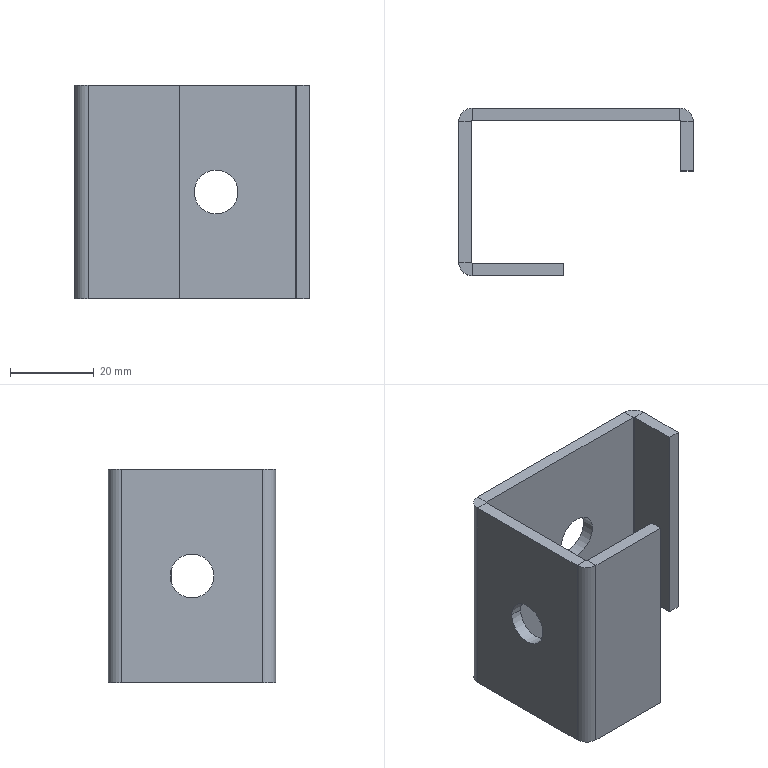Part | SolidWorks | features ICE 2, FlatPattern 1, SMBaseFlange 1, SheetMetal 1 | 1 solid | 34 faces | box 56 x 40 x 51 mm | volume 18577 mm3 | plane 24 | cylinder 10 | commonest cylinder face diameters 10.5 x4 0.4 x3 6.4 x3
STEP:
#1=CARTESIAN_POINT('',(33.75,-3.,30.75));
#2=VERTEX_POINT('',#1);
#3=CARTESIAN_POINT('',(33.75,-3.,20.25));
#4=VERTEX_POINT('',#3);
#5=CARTESIAN_POINT('',(33.75,-3.,25.5));
#6=DIRECTION('',(0.,-1.,0.));
#7=DIRECTION('',(0.,0.,-1.));
#8=AXIS2_PLACEMENT_3D('',#5,#6,#7);
#9=CIRCLE('',#8,5.25);
#10=EDGE_CURVE('',#2,#4,#9,.T.);
#11=ORIENTED_EDGE('',*,*,#10,.T.);
#12=CARTESIAN_POINT('',(33.75,0.,20.25));
#13=VERTEX_POINT('',#12);
#14=CARTESIAN_POINT('',(33.75,-10.,20.25));
#15=DIRECTION('',(0.,1.,0.));
#16=VECTOR('',#15,1000.);
#17=LINE('',#14,#16);
#18=EDGE_CURVE('',#4,#13,#17,.T.);
#19=ORIENTED_EDGE('',*,*,#18,.T.);
#20=CARTESIAN_POINT('',(33.75,0.,30.75));
#21=VERTEX_POINT('',#20);
#22=CARTESIAN_POINT('',(33.75,0.,25.5));
#23=DIRECTION('',(0.,1.,0.));
#24=DIRECTION('',(0.,0.,1.));
#25=AXIS2_PLACEMENT_3D('',#22,#23,#24);
#26=CIRCLE('',#25,5.25);
#27=EDGE_CURVE('',#13,#21,#26,.T.);
#28=ORIENTED_EDGE('',*,*,#27,.T.);
#29=CARTESIAN_POINT('',(33.75,-10.,30.75));
#30=DIRECTION('',(0.,1.,0.));
#31=VECTOR('',#30,1000.);
#32=LINE('',#29,#31);
#33=EDGE_CURVE('',#2,#21,#32,.T.);
#34=ORIENTED_EDGE('',*,*,#33,.F.);
#35=EDGE_LOOP('',(#11,#19,#28,#34));
#36=FACE_OUTER_BOUND('',#35,.T.);
#37=CARTESIAN_POINT('',(33.75,-10.,25.5));
#38=DIRECTION('',(0.,1.,0.));
#39=DIRECTION('',(0.,0.,1.));
#40=AXIS2_PLACEMENT_3D('',#37,#38,#39);
#41=CYLINDRICAL_SURFACE('',#40,5.25);
#42=ADVANCED_FACE('',(#36),#41,.F.);
#43=CARTESIAN_POINT('',(3.,-25.25,25.5));
#44=VERTEX_POINT('',#43);
#45=CARTESIAN_POINT('',(3.,-14.75,25.5));
#46=VERTEX_POINT('',#45);
#47=CARTESIAN_POINT('',(3.,-20.,25.5));
#48=DIRECTION('',(1.,0.,0.));
#49=DIRECTION('',(0.,1.,0.));
#50=AXIS2_PLACEMENT_3D('',#47,#48,#49);
#51=CIRCLE('',#50,5.25);
#52=EDGE_CURVE('',#44,#46,#51,.T.);
#53=ORIENTED_EDGE('',*,*,#52,.T.);
#54=CARTESIAN_POINT('',(0.,-14.75,25.5));
#55=VERTEX_POINT('',#54);
#56=CARTESIAN_POINT('',(10.,-14.75,25.5));
#57=DIRECTION('',(-1.,0.,0.));
#58=VECTOR('',#57,1000.);
#59=LINE('',#56,#58);
#60=EDGE_CURVE('',#46,#55,#59,.T.);
#61=ORIENTED_EDGE('',*,*,#60,.T.);
#62=CARTESIAN_POINT('',(0.,-25.25,25.5));
#63=VERTEX_POINT('',#62);
#64=CARTESIAN_POINT('',(0.,-20.,25.5));
#65=DIRECTION('',(-1.,0.,0.));
#66=DIRECTION('',(0.,-1.,0.));
#67=AXIS2_PLACEMENT_3D('',#64,#65,#66);
#68=CIRCLE('',#67,5.25);
#69=EDGE_CURVE('',#55,#63,#68,.T.);
#70=ORIENTED_EDGE('',*,*,#69,.T.);
#71=CARTESIAN_POINT('',(10.,-25.25,25.5));
#72=DIRECTION('',(-1.,0.,0.));
#73=VECTOR('',#72,1000.);
#74=LINE('',#71,#73);
#75=EDGE_CURVE('',#44,#63,#74,.T.);
#76=ORIENTED_EDGE('',*,*,#75,.F.);
#77=EDGE_LOOP('',(#53,#61,#70,#76));
#78=FACE_OUTER_BOUND('',#77,.T.);
#79=CARTESIAN_POINT('',(10.,-20.,25.5));
#80=DIRECTION('',(-1.,0.,0.));
#81=DIRECTION('',(0.,-1.,0.));
#82=AXIS2_PLACEMENT_3D('',#79,#80,#81);
#83=CYLINDRICAL_SURFACE('',#82,5.25);
#84=ADVANCED_FACE('',(#78),#83,.F.);
#85=CARTESIAN_POINT('',(56.,-3.2,51.));
#86=VERTEX_POINT('',#85);
#87=CARTESIAN_POINT('',(53.,-3.2,51.));
#88=VERTEX_POINT('',#87);
#89=CARTESIAN_POINT('',(56.,-3.2,51.));
#90=DIRECTION('',(-1.,0.,0.));
#91=VECTOR('',#90,1000.);
#92=LINE('',#89,#91);
#93=EDGE_CURVE('',#86,#88,#92,.T.);
#94=ORIENTED_EDGE('',*,*,#93,.F.);
#95=CARTESIAN_POINT('',(52.8,0.,51.));
#96=VERTEX_POINT('',#95);
#97=CARTESIAN_POINT('',(52.8,-3.2,51.));
#98=DIRECTION('',(0.,0.,1.));
#99=DIRECTION('',(-1.,0.,0.));
#100=AXIS2_PLACEMENT_3D('',#97,#98,#99);
#101=CIRCLE('',#100,3.2);
#102=EDGE_CURVE('',#86,#96,#101,.T.);
#103=ORIENTED_EDGE('',*,*,#102,.T.);
#104=CARTESIAN_POINT('',(52.8,-3.,51.));
#105=VERTEX_POINT('',#104);
#106=CARTESIAN_POINT('',(52.8,-3.,51.));
#107=DIRECTION('',(0.,1.,0.));
#108=VECTOR('',#107,1000.);
#109=LINE('',#106,#108);
#110=EDGE_CURVE('',#105,#96,#109,.T.);
#111=ORIENTED_EDGE('',*,*,#110,.F.);
#112=CARTESIAN_POINT('',(52.8,-3.2,51.));
#113=DIRECTION('',(0.,0.,1.));
#114=DIRECTION('',(1.,0.,0.));
#115=AXIS2_PLACEMENT_3D('',#112,#113,#114);
#116=CIRCLE('',#115,0.2);
#117=EDGE_CURVE('',#88,#105,#116,.T.);
#118=ORIENTED_EDGE('',*,*,#117,.F.);
#119=EDGE_LOOP('',(#94,#103,#111,#118));
#120=FACE_OUTER_BOUND('',#119,.T.);
#121=CARTESIAN_POINT('',(56.,-3.2,51.));
#122=DIRECTION('',(0.,0.,1.));
#123=DIRECTION('',(1.,0.,0.));
#124=AXIS2_PLACEMENT_3D('',#121,#122,#123);
#125=PLANE('',#124);
#126=ADVANCED_FACE('',(#120),#125,.T.);
#127=CARTESIAN_POINT('',(56.,-15.,51.));
#128=VERTEX_POINT('',#127);
#129=CARTESIAN_POINT('',(56.,0.,51.));
#130=DIRECTION('',(0.,1.,0.));
#131=VECTOR('',#130,1000.);
#132=LINE('',#129,#131);
#133=EDGE_CURVE('',#128,#86,#132,.T.);
#134=ORIENTED_EDGE('',*,*,#133,.T.);
#135=ORIENTED_EDGE('',*,*,#93,.T.);
#136=CARTESIAN_POINT('',(53.,-15.,51.));
#137=VERTEX_POINT('',#136);
#138=CARTESIAN_POINT('',(53.,0.,51.));
#139=DIRECTION('',(0.,1.,0.));
#140=VECTOR('',#139,1000.);
#141=LINE('',#138,#140);
#142=EDGE_CURVE('',#137,#88,#141,.T.);
#143=ORIENTED_EDGE('',*,*,#142,.F.);
#144=CARTESIAN_POINT('',(56.,-15.,51.));
#145=DIRECTION('',(-1.,0.,0.));
#146=VECTOR('',#145,1000.);
#147=LINE('',#144,#146);
#148=EDGE_CURVE('',#128,#137,#147,.T.);
#149=ORIENTED_EDGE('',*,*,#148,.F.);
#150=EDGE_LOOP('',(#134,#135,#143,#149));
#151=FACE_OUTER_BOUND('',#150,.T.);
#152=CARTESIAN_POINT('',(52.8,-3.,51.));
#153=DIRECTION('',(0.,0.,1.));
#154=DIRECTION('',(1.,0.,0.));
#155=AXIS2_PLACEMENT_3D('',#152,#153,#154);
#156=PLANE('',#155);
#157=ADVANCED_FACE('',(#151),#156,.T.);
#158=CARTESIAN_POINT('',(52.8,0.,0.));
#159=VERTEX_POINT('',#158);
#160=CARTESIAN_POINT('',(52.8,-3.,0.));
#161=VERTEX_POINT('',#160);
#162=CARTESIAN_POINT('',(52.8,0.,0.));
#163=DIRECTION('',(0.,-1.,0.));
#164=VECTOR('',#163,1000.);
#165=LINE('',#162,#164);
#166=EDGE_CURVE('',#159,#161,#165,.T.);
#167=ORIENTED_EDGE('',*,*,#166,.F.);
#168=CARTESIAN_POINT('',(56.,-3.2,0.));
#169=VERTEX_POINT('',#168);
#170=CARTESIAN_POINT('',(52.8,-3.2,0.));
#171=DIRECTION('',(0.,0.,1.));
#172=DIRECTION('',(-1.,0.,0.));
#173=AXIS2_PLACEMENT_3D('',#170,#171,#172);
#174=CIRCLE('',#173,3.2);
#175=EDGE_CURVE('',#169,#159,#174,.T.);
#176=ORIENTED_EDGE('',*,*,#175,.F.);
#177=CARTESIAN_POINT('',(53.,-3.2,0.));
#178=VERTEX_POINT('',#177);
#179=CARTESIAN_POINT('',(53.,-3.2,0.));
#180=DIRECTION('',(1.,0.,0.));
#181=VECTOR('',#180,1000.);
#182=LINE('',#179,#181);
#183=EDGE_CURVE('',#178,#169,#182,.T.);
#184=ORIENTED_EDGE('',*,*,#183,.F.);
#185=CARTESIAN_POINT('',(52.8,-3.2,0.));
#186=DIRECTION('',(0.,0.,1.));
#187=DIRECTION('',(1.,0.,0.));
#188=AXIS2_PLACEMENT_3D('',#185,#186,#187);
#189=CIRCLE('',#188,0.2);
#190=EDGE_CURVE('',#178,#161,#189,.T.);
#191=ORIENTED_EDGE('',*,*,#190,.T.);
#192=EDGE_LOOP('',(#167,#176,#184,#191));
#193=FACE_OUTER_BOUND('',#192,.T.);
#194=CARTESIAN_POINT('',(52.8,0.,0.));
#195=DIRECTION('',(0.,0.,-1.));
#196=DIRECTION('',(-1.,0.,0.));
#197=AXIS2_PLACEMENT_3D('',#194,#195,#196);
#198=PLANE('',#197);
#199=ADVANCED_FACE('',(#193),#198,.T.);
#200=CARTESIAN_POINT('',(3.2,0.,0.));
#201=VERTEX_POINT('',#200);
#202=CARTESIAN_POINT('',(0.,0.,0.));
#203=DIRECTION('',(-1.,0.,0.));
#204=VECTOR('',#203,1000.);
#205=LINE('',#202,#204);
#206=EDGE_CURVE('',#159,#201,#205,.T.);
#207=ORIENTED_EDGE('',*,*,#206,.F.);
#208=ORIENTED_EDGE('',*,*,#166,.T.);
#209=CARTESIAN_POINT('',(3.2,-3.,0.));
#210=VERTEX_POINT('',#209);
#211=CARTESIAN_POINT('',(0.,-3.,0.));
#212=DIRECTION('',(-1.,0.,0.));
#213=VECTOR('',#212,1000.);
#214=LINE('',#211,#213);
#215=EDGE_CURVE('',#161,#210,#214,.T.);
#216=ORIENTED_EDGE('',*,*,#215,.T.);
#217=CARTESIAN_POINT('',(3.2,-3.,0.));
#218=DIRECTION('',(0.,1.,0.));
#219=VECTOR('',#218,1000.);
#220=LINE('',#217,#219);
#221=EDGE_CURVE('',#210,#201,#220,.T.);
#222=ORIENTED_EDGE('',*,*,#221,.T.);
#223=EDGE_LOOP('',(#207,#208,#216,#222));
#224=FACE_OUTER_BOUND('',#223,.T.);
#225=CARTESIAN_POINT('',(53.,-3.2,0.));
#226=DIRECTION('',(0.,0.,-1.));
#227=DIRECTION('',(-1.,0.,0.));
#228=AXIS2_PLACEMENT_3D('',#225,#226,#227);
#229=PLANE('',#228);
#230=ADVANCED_FACE('',(#224),#229,.T.);
#231=CARTESIAN_POINT('',(3.2,0.,51.));
#232=VERTEX_POINT('',#231);
#233=CARTESIAN_POINT('',(3.2,-3.,51.));
#234=VERTEX_POINT('',#233);
#235=CARTESIAN_POINT('',(3.2,0.,51.));
#236=DIRECTION('',(0.,-1.,0.));
#237=VECTOR('',#236,1000.);
#238=LINE('',#235,#237);
#239=EDGE_CURVE('',#232,#234,#238,.T.);
#240=ORIENTED_EDGE('',*,*,#239,.F.);
#241=CARTESIAN_POINT('',(0.,-3.2,51.));
#242=VERTEX_POINT('',#241);
#243=CARTESIAN_POINT('',(3.2,-3.2,51.));
#244=DIRECTION('',(0.,0.,1.));
#245=DIRECTION('',(-1.,0.,0.));
#246=AXIS2_PLACEMENT_3D('',#243,#244,#245);
#247=CIRCLE('',#246,3.2);
#248=EDGE_CURVE('',#232,#242,#247,.T.);
#249=ORIENTED_EDGE('',*,*,#248,.T.);
#250=CARTESIAN_POINT('',(3.,-3.2,51.));
#251=VERTEX_POINT('',#250);
#252=CARTESIAN_POINT('',(3.,-3.2,51.));
#253=DIRECTION('',(-1.,0.,0.));
#254=VECTOR('',#253,1000.);
#255=LINE('',#252,#254);
#256=EDGE_CURVE('',#251,#242,#255,.T.);
#257=ORIENTED_EDGE('',*,*,#256,.F.);
#258=CARTESIAN_POINT('',(3.2,-3.2,51.));
#259=DIRECTION('',(0.,0.,1.));
#260=DIRECTION('',(1.,0.,0.));
#261=AXIS2_PLACEMENT_3D('',#258,#259,#260);
#262=CIRCLE('',#261,0.2);
#263=EDGE_CURVE('',#234,#251,#262,.T.);
#264=ORIENTED_EDGE('',*,*,#263,.F.);
#265=EDGE_LOOP('',(#240,#249,#257,#264));
#266=FACE_OUTER_BOUND('',#265,.T.);
#267=CARTESIAN_POINT('',(3.2,0.,51.));
#268=DIRECTION('',(0.,0.,1.));
#269=DIRECTION('',(1.,0.,0.));
#270=AXIS2_PLACEMENT_3D('',#267,#268,#269);
#271=PLANE('',#270);
#272=ADVANCED_FACE('',(#266),#271,.T.);
#273=CARTESIAN_POINT('',(0.,0.,51.));
#274=DIRECTION('',(-1.,0.,0.));
#275=VECTOR('',#274,1000.);
#276=LINE('',#273,#275);
#277=EDGE_CURVE('',#96,#232,#276,.T.);
#278=ORIENTED_EDGE('',*,*,#277,.T.);
#279=ORIENTED_EDGE('',*,*,#239,.T.);
#280=CARTESIAN_POINT('',(0.,-3.,51.));
#281=DIRECTION('',(-1.,0.,0.));
#282=VECTOR('',#281,1000.);
#283=LINE('',#280,#282);
#284=EDGE_CURVE('',#105,#234,#283,.T.);
#285=ORIENTED_EDGE('',*,*,#284,.F.);
#286=ORIENTED_EDGE('',*,*,#110,.T.);
#287=EDGE_LOOP('',(#278,#279,#285,#286));
#288=FACE_OUTER_BOUND('',#287,.T.);
#289=CARTESIAN_POINT('',(3.,-3.2,51.));
#290=DIRECTION('',(0.,0.,1.));
#291=DIRECTION('',(1.,0.,0.));
#292=AXIS2_PLACEMENT_3D('',#289,#290,#291);
#293=PLANE('',#292);
#294=ADVANCED_FACE('',(#288),#293,.T.);
#295=CARTESIAN_POINT('',(0.,-3.2,0.));
#296=VERTEX_POINT('',#295);
#297=CARTESIAN_POINT('',(3.,-3.2,0.));
#298=VERTEX_POINT('',#297);
#299=CARTESIAN_POINT('',(0.,-3.2,0.));
#300=DIRECTION('',(1.,0.,0.));
#301=VECTOR('',#300,1000.);
#302=LINE('',#299,#301);
#303=EDGE_CURVE('',#296,#298,#302,.T.);
#304=ORIENTED_EDGE('',*,*,#303,.F.);
#305=CARTESIAN_POINT('',(3.2,-3.2,0.));
#306=DIRECTION('',(0.,0.,1.));
#307=DIRECTION('',(-1.,0.,0.));
#308=AXIS2_PLACEMENT_3D('',#305,#306,#307);
#309=CIRCLE('',#308,3.2);
#310=EDGE_CURVE('',#201,#296,#309,.T.);
#311=ORIENTED_EDGE('',*,*,#310,.F.);
#312=ORIENTED_EDGE('',*,*,#221,.F.);
#313=CARTESIAN_POINT('',(3.2,-3.2,0.));
#314=DIRECTION('',(0.,0.,1.));
#315=DIRECTION('',(1.,0.,0.));
#316=AXIS2_PLACEMENT_3D('',#313,#314,#315);
#317=CIRCLE('',#316,0.2);
#318=EDGE_CURVE('',#210,#298,#317,.T.);
#319=ORIENTED_EDGE('',*,*,#318,.T.);
#320=EDGE_LOOP('',(#304,#311,#312,#319));
#321=FACE_OUTER_BOUND('',#320,.T.);
#322=CARTESIAN_POINT('',(0.,-3.2,0.));
#323=DIRECTION('',(0.,0.,-1.));
#324=DIRECTION('',(-1.,0.,0.));
#325=AXIS2_PLACEMENT_3D('',#322,#323,#324);
#326=PLANE('',#325);
#327=ADVANCED_FACE('',(#321),#326,.T.);
#328=CARTESIAN_POINT('',(0.,-36.8,0.));
#329=VERTEX_POINT('',#328);
#330=CARTESIAN_POINT('',(0.,0.,0.));
#331=DIRECTION('',(0.,-1.,0.));
#332=VECTOR('',#331,1000.);
#333=LINE('',#330,#332);
#334=EDGE_CURVE('',#296,#329,#333,.T.);
#335=ORIENTED_EDGE('',*,*,#334,.F.);
#336=ORIENTED_EDGE('',*,*,#303,.T.);
#337=CARTESIAN_POINT('',(3.,-36.8,0.));
#338=VERTEX_POINT('',#337);
#339=CARTESIAN_POINT('',(3.,0.,0.));
#340=DIRECTION('',(0.,-1.,0.));
#341=VECTOR('',#340,1000.);
#342=LINE('',#339,#341);
#343=EDGE_CURVE('',#298,#338,#342,.T.);
#344=ORIENTED_EDGE('',*,*,#343,.T.);
#345=CARTESIAN_POINT('',(3.,-36.8,0.));
#346=DIRECTION('',(-1.,0.,0.));
#347=VECTOR('',#346,1000.);
#348=LINE('',#345,#347);
#349=EDGE_CURVE('',#338,#329,#348,.T.);
#350=ORIENTED_EDGE('',*,*,#349,.T.);
#351=EDGE_LOOP('',(#335,#336,#344,#350));
#352=FACE_OUTER_BOUND('',#351,.T.);
#353=CARTESIAN_POINT('',(3.2,-3.,0.));
#354=DIRECTION('',(0.,0.,-1.));
#355=DIRECTION('',(-1.,0.,0.));
#356=AXIS2_PLACEMENT_3D('',#353,#354,#355);
#357=PLANE('',#356);
#358=ADVANCED_FACE('',(#352),#357,.T.);
#359=CARTESIAN_POINT('',(0.,-36.8,51.));
#360=VERTEX_POINT('',#359);
#361=CARTESIAN_POINT('',(3.,-36.8,51.));
#362=VERTEX_POINT('',#361);
#363=CARTESIAN_POINT('',(0.,-36.8,51.));
#364=DIRECTION('',(1.,0.,0.));
#365=VECTOR('',#364,1000.);
#366=LINE('',#363,#365);
#367=EDGE_CURVE('',#360,#362,#366,.T.);
#368=ORIENTED_EDGE('',*,*,#367,.F.);
#369=CARTESIAN_POINT('',(3.2,-40.,51.));
#370=VERTEX_POINT('',#369);
#371=CARTESIAN_POINT('',(3.2,-36.8,51.));
#372=DIRECTION('',(0.,0.,1.));
#373=DIRECTION('',(-1.,0.,0.));
#374=AXIS2_PLACEMENT_3D('',#371,#372,#373);
#375=CIRCLE('',#374,3.2);
#376=EDGE_CURVE('',#360,#370,#375,.T.);
#377=ORIENTED_EDGE('',*,*,#376,.T.);
#378=CARTESIAN_POINT('',(3.2,-37.,51.));
#379=VERTEX_POINT('',#378);
#380=CARTESIAN_POINT('',(3.2,-37.,51.));
#381=DIRECTION('',(0.,-1.,0.));
#382=VECTOR('',#381,1000.);
#383=LINE('',#380,#382);
#384=EDGE_CURVE('',#379,#370,#383,.T.);
#385=ORIENTED_EDGE('',*,*,#384,.F.);
#386=CARTESIAN_POINT('',(3.2,-36.8,51.));
#387=DIRECTION('',(0.,0.,1.));
#388=DIRECTION('',(1.,0.,0.));
#389=AXIS2_PLACEMENT_3D('',#386,#387,#388);
#390=CIRCLE('',#389,0.2);
#391=EDGE_CURVE('',#362,#379,#390,.T.);
#392=ORIENTED_EDGE('',*,*,#391,.F.);
#393=EDGE_LOOP('',(#368,#377,#385,#392));
#394=FACE_OUTER_BOUND('',#393,.T.);
#395=CARTESIAN_POINT('',(0.,-36.8,51.));
#396=DIRECTION('',(0.,0.,1.));
#397=DIRECTION('',(1.,0.,0.));
#398=AXIS2_PLACEMENT_3D('',#395,#396,#397);
#399=PLANE('',#398);
#400=ADVANCED_FACE('',(#394),#399,.T.);
#401=CARTESIAN_POINT('',(0.,0.,51.));
#402=DIRECTION('',(0.,-1.,0.));
#403=VECTOR('',#402,1000.);
#404=LINE('',#401,#403);
#405=EDGE_CURVE('',#242,#360,#404,.T.);
#406=ORIENTED_EDGE('',*,*,#405,.T.);
#407=ORIENTED_EDGE('',*,*,#367,.T.);
#408=CARTESIAN_POINT('',(3.,0.,51.));
#409=DIRECTION('',(0.,-1.,0.));
#410=VECTOR('',#409,1000.);
#411=LINE('',#408,#410);
#412=EDGE_CURVE('',#251,#362,#411,.T.);
#413=ORIENTED_EDGE('',*,*,#412,.F.);
#414=ORIENTED_EDGE('',*,*,#256,.T.);
#415=EDGE_LOOP('',(#406,#407,#413,#414));
#416=FACE_OUTER_BOUND('',#415,.T.);
#417=CARTESIAN_POINT('',(3.2,-37.,51.));
#418=DIRECTION('',(0.,0.,1.));
#419=DIRECTION('',(1.,0.,0.));
#420=AXIS2_PLACEMENT_3D('',#417,#418,#419);
#421=PLANE('',#420);
#422=ADVANCED_FACE('',(#416),#421,.T.);
#423=CARTESIAN_POINT('',(3.2,-40.,0.));
#424=VERTEX_POINT('',#423);
#425=CARTESIAN_POINT('',(3.2,-37.,0.));
#426=VERTEX_POINT('',#425);
#427=CARTESIAN_POINT('',(3.2,-40.,0.));
#428=DIRECTION('',(0.,1.,0.));
#429=VECTOR('',#428,1000.);
#430=LINE('',#427,#429);
#431=EDGE_CURVE('',#424,#426,#430,.T.);
#432=ORIENTED_EDGE('',*,*,#431,.F.);
#433=CARTESIAN_POINT('',(3.2,-36.8,0.));
#434=DIRECTION('',(0.,0.,1.));
#435=DIRECTION('',(-1.,0.,0.));
#436=AXIS2_PLACEMENT_3D('',#433,#434,#435);
#437=CIRCLE('',#436,3.2);
#438=EDGE_CURVE('',#329,#424,#437,.T.);
#439=ORIENTED_EDGE('',*,*,#438,.F.);
#440=ORIENTED_EDGE('',*,*,#349,.F.);
#441=CARTESIAN_POINT('',(3.2,-36.8,0.));
#442=DIRECTION('',(0.,0.,1.));
#443=DIRECTION('',(1.,0.,0.));
#444=AXIS2_PLACEMENT_3D('',#441,#442,#443);
#445=CIRCLE('',#444,0.2);
#446=EDGE_CURVE('',#338,#426,#445,.T.);
#447=ORIENTED_EDGE('',*,*,#446,.T.);
#448=EDGE_LOOP('',(#432,#439,#440,#447));
#449=FACE_OUTER_BOUND('',#448,.T.);
#450=CARTESIAN_POINT('',(3.2,-40.,0.));
#451=DIRECTION('',(0.,0.,-1.));
#452=DIRECTION('',(-1.,0.,0.));
#453=AXIS2_PLACEMENT_3D('',#450,#451,#452);
#454=PLANE('',#453);
#455=ADVANCED_FACE('',(#449),#454,.T.);
#456=CARTESIAN_POINT('',(25.,-40.,0.));
#457=VERTEX_POINT('',#456);
#458=CARTESIAN_POINT('',(0.,-40.,0.));
#459=DIRECTION('',(1.,0.,0.));
#460=VECTOR('',#459,1000.);
#461=LINE('',#458,#460);
#462=EDGE_CURVE('',#424,#457,#461,.T.);
#463=ORIENTED_EDGE('',*,*,#462,.F.);
#464=ORIENTED_EDGE('',*,*,#431,.T.);
#465=CARTESIAN_POINT('',(25.,-37.,0.));
#466=VERTEX_POINT('',#465);
#467=CARTESIAN_POINT('',(0.,-37.,0.));
#468=DIRECTION('',(1.,0.,0.));
#469=VECTOR('',#468,1000.);
#470=LINE('',#467,#469);
#471=EDGE_CURVE('',#426,#466,#470,.T.);
#472=ORIENTED_EDGE('',*,*,#471,.T.);
#473=CARTESIAN_POINT('',(25.,-37.,0.));
#474=DIRECTION('',(0.,-1.,0.));
#475=VECTOR('',#474,1000.);
#476=LINE('',#473,#475);
#477=EDGE_CURVE('',#466,#457,#476,.T.);
#478=ORIENTED_EDGE('',*,*,#477,.T.);
#479=EDGE_LOOP('',(#463,#464,#472,#478));
#480=FACE_OUTER_BOUND('',#479,.T.);
#481=CARTESIAN_POINT('',(3.,-36.8,0.));
#482=DIRECTION('',(0.,0.,-1.));
#483=DIRECTION('',(-1.,0.,0.));
#484=AXIS2_PLACEMENT_3D('',#481,#482,#483);
#485=PLANE('',#484);
#486=ADVANCED_FACE('',(#480),#485,.T.);
#487=ORIENTED_EDGE('',*,*,#462,.T.);
#488=CARTESIAN_POINT('',(25.,-40.,51.));
#489=VERTEX_POINT('',#488);
#490=CARTESIAN_POINT('',(25.,-40.,51.));
#491=DIRECTION('',(0.,0.,-1.));
#492=VECTOR('',#491,1000.);
#493=LINE('',#490,#492);
#494=EDGE_CURVE('',#489,#457,#493,.T.);
#495=ORIENTED_EDGE('',*,*,#494,.F.);
#496=CARTESIAN_POINT('',(0.,-40.,51.));
#497=DIRECTION('',(1.,0.,0.));
#498=VECTOR('',#497,1000.);
#499=LINE('',#496,#498);
#500=EDGE_CURVE('',#370,#489,#499,.T.);
#501=ORIENTED_EDGE('',*,*,#500,.F.);
#502=CARTESIAN_POINT('',(3.2,-40.,51.));
#503=DIRECTION('',(0.,0.,-1.));
#504=VECTOR('',#503,1000.);
#505=LINE('',#502,#504);
#506=EDGE_CURVE('',#370,#424,#505,.T.);
#507=ORIENTED_EDGE('',*,*,#506,.T.);
#508=EDGE_LOOP('',(#487,#495,#501,#507));
#509=FACE_OUTER_BOUND('',#508,.T.);
#510=CARTESIAN_POINT('',(0.,-40.,51.));
#511=DIRECTION('',(0.,1.,0.));
#512=DIRECTION('',(0.,0.,1.));
#513=AXIS2_PLACEMENT_3D('',#510,#511,#512);
#514=PLANE('',#513);
#515=ADVANCED_FACE('',(#509),#514,.F.);
#516=ORIENTED_EDGE('',*,*,#477,.F.);
#517=CARTESIAN_POINT('',(25.,-37.,51.));
#518=VERTEX_POINT('',#517);
#519=CARTESIAN_POINT('',(25.,-37.,51.));
#520=DIRECTION('',(0.,0.,-1.));
#521=VECTOR('',#520,1000.);
#522=LINE('',#519,#521);
#523=EDGE_CURVE('',#518,#466,#522,.T.);
#524=ORIENTED_EDGE('',*,*,#523,.F.);
#525=CARTESIAN_POINT('',(25.,-37.,51.));
#526=DIRECTION('',(0.,-1.,0.));
#527=VECTOR('',#526,1000.);
#528=LINE('',#525,#527);
#529=EDGE_CURVE('',#518,#489,#528,.T.);
#530=ORIENTED_EDGE('',*,*,#529,.T.);
#531=ORIENTED_EDGE('',*,*,#494,.T.);
#532=EDGE_LOOP('',(#516,#524,#530,#531));
#533=FACE_OUTER_BOUND('',#532,.T.);
#534=CARTESIAN_POINT('',(25.,-37.,51.));
#535=DIRECTION('',(1.,0.,0.));
#536=DIRECTION('',(0.,0.,-1.));
#537=AXIS2_PLACEMENT_3D('',#534,#535,#536);
#538=PLANE('',#537);
#539=ADVANCED_FACE('',(#533),#538,.T.);
#540=ORIENTED_EDGE('',*,*,#471,.F.);
#541=CARTESIAN_POINT('',(3.2,-37.,51.));
#542=DIRECTION('',(0.,0.,-1.));
#543=VECTOR('',#542,1000.);
#544=LINE('',#541,#543);
#545=EDGE_CURVE('',#379,#426,#544,.T.);
#546=ORIENTED_EDGE('',*,*,#545,.F.);
#547=CARTESIAN_POINT('',(0.,-37.,51.));
#548=DIRECTION('',(1.,0.,0.));
#549=VECTOR('',#548,1000.);
#550=LINE('',#547,#549);
#551=EDGE_CURVE('',#379,#518,#550,.T.);
#552=ORIENTED_EDGE('',*,*,#551,.T.);
#553=ORIENTED_EDGE('',*,*,#523,.T.);
#554=EDGE_LOOP('',(#540,#546,#552,#553));
#555=FACE_OUTER_BOUND('',#554,.T.);
#556=CARTESIAN_POINT('',(0.,-37.,51.));
#557=DIRECTION('',(0.,1.,0.));
#558=DIRECTION('',(0.,0.,1.));
#559=AXIS2_PLACEMENT_3D('',#556,#557,#558);
#560=PLANE('',#559);
#561=ADVANCED_FACE('',(#555),#560,.T.);
#562=ORIENTED_EDGE('',*,*,#446,.F.);
#563=CARTESIAN_POINT('',(3.,-36.8,51.));
#564=DIRECTION('',(0.,0.,-1.));
#565=VECTOR('',#564,1000.);
#566=LINE('',#563,#565);
#567=EDGE_CURVE('',#362,#338,#566,.T.);
#568=ORIENTED_EDGE('',*,*,#567,.F.);
#569=ORIENTED_EDGE('',*,*,#391,.T.);
#570=ORIENTED_EDGE('',*,*,#545,.T.);
#571=EDGE_LOOP('',(#562,#568,#569,#570));
#572=FACE_OUTER_BOUND('',#571,.T.);
#573=CARTESIAN_POINT('',(3.2,-36.8,51.));
#574=DIRECTION('',(0.,0.,-1.));
#575=DIRECTION('',(-1.,0.,0.));
#576=AXIS2_PLACEMENT_3D('',#573,#574,#575);
#577=CYLINDRICAL_SURFACE('',#576,0.2);
#578=ADVANCED_FACE('',(#572),#577,.F.);
#579=ORIENTED_EDGE('',*,*,#52,.F.);
#580=CARTESIAN_POINT('',(3.,-20.,25.5));
#581=DIRECTION('',(1.,0.,0.));
#582=DIRECTION('',(0.,1.,0.));
#583=AXIS2_PLACEMENT_3D('',#580,#581,#582);
#584=CIRCLE('',#583,5.25);
#585=EDGE_CURVE('',#46,#44,#584,.T.);
#586=ORIENTED_EDGE('',*,*,#585,.F.);
#587=EDGE_LOOP('',(#579,#586));
#588=FACE_BOUND('',#587,.T.);
#589=ORIENTED_EDGE('',*,*,#343,.F.);
#590=CARTESIAN_POINT('',(3.,-3.2,51.));
#591=DIRECTION('',(0.,0.,-1.));
#592=VECTOR('',#591,1000.);
#593=LINE('',#590,#592);
#594=EDGE_CURVE('',#251,#298,#593,.T.);
#595=ORIENTED_EDGE('',*,*,#594,.F.);
#596=ORIENTED_EDGE('',*,*,#412,.T.);
#597=ORIENTED_EDGE('',*,*,#567,.T.);
#598=EDGE_LOOP('',(#589,#595,#596,#597));
#599=FACE_OUTER_BOUND('',#598,.T.);
#600=CARTESIAN_POINT('',(3.,0.,51.));
#601=DIRECTION('',(1.,0.,0.));
#602=DIRECTION('',(0.,1.,0.));
#603=AXIS2_PLACEMENT_3D('',#600,#601,#602);
#604=PLANE('',#603);
#605=ADVANCED_FACE('',(#588,#599),#604,.T.);
#606=ORIENTED_EDGE('',*,*,#318,.F.);
#607=CARTESIAN_POINT('',(3.2,-3.,51.));
#608=DIRECTION('',(0.,0.,-1.));
#609=VECTOR('',#608,1000.);
#610=LINE('',#607,#609);
#611=EDGE_CURVE('',#234,#210,#610,.T.);
#612=ORIENTED_EDGE('',*,*,#611,.F.);
#613=ORIENTED_EDGE('',*,*,#263,.T.);
#614=ORIENTED_EDGE('',*,*,#594,.T.);
#615=EDGE_LOOP('',(#606,#612,#613,#614));
#616=FACE_OUTER_BOUND('',#615,.T.);
#617=CARTESIAN_POINT('',(3.2,-3.2,51.));
#618=DIRECTION('',(0.,0.,-1.));
#619=DIRECTION('',(-1.,0.,0.));
#620=AXIS2_PLACEMENT_3D('',#617,#618,#619);
#621=CYLINDRICAL_SURFACE('',#620,0.2);
#622=ADVANCED_FACE('',(#616),#621,.F.);
#623=ORIENTED_EDGE('',*,*,#10,.F.);
#624=CARTESIAN_POINT('',(33.75,-3.,25.5));
#625=DIRECTION('',(0.,-1.,0.));
#626=DIRECTION('',(0.,0.,-1.));
#627=AXIS2_PLACEMENT_3D('',#624,#625,#626);
#628=CIRCLE('',#627,5.25);
#629=EDGE_CURVE('',#4,#2,#628,.T.);
#630=ORIENTED_EDGE('',*,*,#629,.F.);
#631=EDGE_LOOP('',(#623,#630));
#632=FACE_BOUND('',#631,.T.);
#633=ORIENTED_EDGE('',*,*,#215,.F.);
#634=CARTESIAN_POINT('',(52.8,-3.,51.));
#635=DIRECTION('',(0.,0.,-1.));
#636=VECTOR('',#635,1000.);
#637=LINE('',#634,#636);
#638=EDGE_CURVE('',#105,#161,#637,.T.);
#639=ORIENTED_EDGE('',*,*,#638,.F.);
#640=ORIENTED_EDGE('',*,*,#284,.T.);
#641=ORIENTED_EDGE('',*,*,#611,.T.);
#642=EDGE_LOOP('',(#633,#639,#640,#641));
#643=FACE_OUTER_BOUND('',#642,.T.);
#644=CARTESIAN_POINT('',(0.,-3.,51.));
#645=DIRECTION('',(0.,-1.,0.));
#646=DIRECTION('',(0.,0.,-1.));
#647=AXIS2_PLACEMENT_3D('',#644,#645,#646);
#648=PLANE('',#647);
#649=ADVANCED_FACE('',(#632,#643),#648,.T.);
#650=ORIENTED_EDGE('',*,*,#190,.F.);
#651=CARTESIAN_POINT('',(53.,-3.2,51.));
#652=DIRECTION('',(0.,0.,-1.));
#653=VECTOR('',#652,1000.);
#654=LINE('',#651,#653);
#655=EDGE_CURVE('',#88,#178,#654,.T.);
#656=ORIENTED_EDGE('',*,*,#655,.F.);
#657=ORIENTED_EDGE('',*,*,#117,.T.);
#658=ORIENTED_EDGE('',*,*,#638,.T.);
#659=EDGE_LOOP('',(#650,#656,#657,#658));
#660=FACE_OUTER_BOUND('',#659,.T.);
#661=CARTESIAN_POINT('',(52.8,-3.2,51.));
#662=DIRECTION('',(0.,0.,-1.));
#663=DIRECTION('',(-1.,0.,0.));
#664=AXIS2_PLACEMENT_3D('',#661,#662,#663);
#665=CYLINDRICAL_SURFACE('',#664,0.2);
#666=ADVANCED_FACE('',(#660),#665,.F.);
#667=CARTESIAN_POINT('',(53.,-15.,0.));
#668=VERTEX_POINT('',#667);
#669=CARTESIAN_POINT('',(53.,0.,0.));
#670=DIRECTION('',(0.,1.,0.));
#671=VECTOR('',#670,1000.);
#672=LINE('',#669,#671);
#673=EDGE_CURVE('',#668,#178,#672,.T.);
#674=ORIENTED_EDGE('',*,*,#673,.F.);
#675=CARTESIAN_POINT('',(53.,-15.,51.));
#676=DIRECTION('',(0.,0.,-1.));
#677=VECTOR('',#676,1000.);
#678=LINE('',#675,#677);
#679=EDGE_CURVE('',#137,#668,#678,.T.);
#680=ORIENTED_EDGE('',*,*,#679,.F.);
#681=ORIENTED_EDGE('',*,*,#142,.T.);
#682=ORIENTED_EDGE('',*,*,#655,.T.);
#683=EDGE_LOOP('',(#674,#680,#681,#682));
#684=FACE_OUTER_BOUND('',#683,.T.);
#685=CARTESIAN_POINT('',(53.,0.,51.));
#686=DIRECTION('',(-1.,0.,0.));
#687=DIRECTION('',(0.,0.,1.));
#688=AXIS2_PLACEMENT_3D('',#685,#686,#687);
#689=PLANE('',#688);
#690=ADVANCED_FACE('',(#684),#689,.T.);
#691=CARTESIAN_POINT('',(56.,-15.,0.));
#692=VERTEX_POINT('',#691);
#693=CARTESIAN_POINT('',(56.,-15.,0.));
#694=DIRECTION('',(-1.,0.,0.));
#695=VECTOR('',#694,1000.);
#696=LINE('',#693,#695);
#697=EDGE_CURVE('',#692,#668,#696,.T.);
#698=ORIENTED_EDGE('',*,*,#697,.F.);
#699=CARTESIAN_POINT('',(56.,-15.,51.));
#700=DIRECTION('',(0.,0.,-1.));
#701=VECTOR('',#700,1000.);
#702=LINE('',#699,#701);
#703=EDGE_CURVE('',#128,#692,#702,.T.);
#704=ORIENTED_EDGE('',*,*,#703,.F.);
#705=ORIENTED_EDGE('',*,*,#148,.T.);
#706=ORIENTED_EDGE('',*,*,#679,.T.);
#707=EDGE_LOOP('',(#698,#704,#705,#706));
#708=FACE_OUTER_BOUND('',#707,.T.);
#709=CARTESIAN_POINT('',(56.,-15.,51.));
#710=DIRECTION('',(0.,-1.,0.));
#711=DIRECTION('',(0.,0.,-1.));
#712=AXIS2_PLACEMENT_3D('',#709,#710,#711);
#713=PLANE('',#712);
#714=ADVANCED_FACE('',(#708),#713,.T.);
#715=CARTESIAN_POINT('',(56.,0.,0.));
#716=DIRECTION('',(0.,1.,0.));
#717=VECTOR('',#716,1000.);
#718=LINE('',#715,#717);
#719=EDGE_CURVE('',#692,#169,#718,.T.);
#720=ORIENTED_EDGE('',*,*,#719,.T.);
#721=CARTESIAN_POINT('',(56.,-3.2,51.));
#722=DIRECTION('',(0.,0.,-1.));
#723=VECTOR('',#722,1000.);
#724=LINE('',#721,#723);
#725=EDGE_CURVE('',#86,#169,#724,.T.);
#726=ORIENTED_EDGE('',*,*,#725,.F.);
#727=ORIENTED_EDGE('',*,*,#133,.F.);
#728=ORIENTED_EDGE('',*,*,#703,.T.);
#729=EDGE_LOOP('',(#720,#726,#727,#728));
#730=FACE_OUTER_BOUND('',#729,.T.);
#731=CARTESIAN_POINT('',(56.,0.,51.));
#732=DIRECTION('',(-1.,0.,0.));
#733=DIRECTION('',(0.,0.,1.));
#734=AXIS2_PLACEMENT_3D('',#731,#732,#733);
#735=PLANE('',#734);
#736=ADVANCED_FACE('',(#730),#735,.F.);
#737=ORIENTED_EDGE('',*,*,#175,.T.);
#738=CARTESIAN_POINT('',(52.8,0.,51.));
#739=DIRECTION('',(0.,0.,-1.));
#740=VECTOR('',#739,1000.);
#741=LINE('',#738,#740);
#742=EDGE_CURVE('',#96,#159,#741,.T.);
#743=ORIENTED_EDGE('',*,*,#742,.F.);
#744=ORIENTED_EDGE('',*,*,#102,.F.);
#745=ORIENTED_EDGE('',*,*,#725,.T.);
#746=EDGE_LOOP('',(#737,#743,#744,#745));
#747=FACE_OUTER_BOUND('',#746,.T.);
#748=CARTESIAN_POINT('',(52.8,-3.2,51.));
#749=DIRECTION('',(0.,0.,-1.));
#750=DIRECTION('',(-1.,0.,0.));
#751=AXIS2_PLACEMENT_3D('',#748,#749,#750);
#752=CYLINDRICAL_SURFACE('',#751,3.2);
#753=ADVANCED_FACE('',(#747),#752,.T.);
#754=CARTESIAN_POINT('',(33.75,0.,25.5));
#755=DIRECTION('',(0.,1.,0.));
#756=DIRECTION('',(0.,0.,1.));
#757=AXIS2_PLACEMENT_3D('',#754,#755,#756);
#758=CIRCLE('',#757,5.25);
#759=EDGE_CURVE('',#21,#13,#758,.T.);
#760=ORIENTED_EDGE('',*,*,#759,.F.);
#761=ORIENTED_EDGE('',*,*,#27,.F.);
#762=EDGE_LOOP('',(#760,#761));
#763=FACE_BOUND('',#762,.T.);
#764=ORIENTED_EDGE('',*,*,#206,.T.);
#765=CARTESIAN_POINT('',(3.2,0.,51.));
#766=DIRECTION('',(0.,0.,-1.));
#767=VECTOR('',#766,1000.);
#768=LINE('',#765,#767);
#769=EDGE_CURVE('',#232,#201,#768,.T.);
#770=ORIENTED_EDGE('',*,*,#769,.F.);
#771=ORIENTED_EDGE('',*,*,#277,.F.);
#772=ORIENTED_EDGE('',*,*,#742,.T.);
#773=EDGE_LOOP('',(#764,#770,#771,#772));
#774=FACE_OUTER_BOUND('',#773,.T.);
#775=CARTESIAN_POINT('',(0.,0.,51.));
#776=DIRECTION('',(0.,-1.,0.));
#777=DIRECTION('',(0.,0.,-1.));
#778=AXIS2_PLACEMENT_3D('',#775,#776,#777);
#779=PLANE('',#778);
#780=ADVANCED_FACE('',(#763,#774),#779,.F.);
#781=ORIENTED_EDGE('',*,*,#310,.T.);
#782=CARTESIAN_POINT('',(0.,-3.2,51.));
#783=DIRECTION('',(0.,0.,-1.));
#784=VECTOR('',#783,1000.);
#785=LINE('',#782,#784);
#786=EDGE_CURVE('',#242,#296,#785,.T.);
#787=ORIENTED_EDGE('',*,*,#786,.F.);
#788=ORIENTED_EDGE('',*,*,#248,.F.);
#789=ORIENTED_EDGE('',*,*,#769,.T.);
#790=EDGE_LOOP('',(#781,#787,#788,#789));
#791=FACE_OUTER_BOUND('',#790,.T.);
#792=CARTESIAN_POINT('',(3.2,-3.2,51.));
#793=DIRECTION('',(0.,0.,-1.));
#794=DIRECTION('',(-1.,0.,0.));
#795=AXIS2_PLACEMENT_3D('',#792,#793,#794);
#796=CYLINDRICAL_SURFACE('',#795,3.2);
#797=ADVANCED_FACE('',(#791),#796,.T.);
#798=CARTESIAN_POINT('',(0.,-20.,25.5));
#799=DIRECTION('',(-1.,0.,0.));
#800=DIRECTION('',(0.,-1.,0.));
#801=AXIS2_PLACEMENT_3D('',#798,#799,#800);
#802=CIRCLE('',#801,5.25);
#803=EDGE_CURVE('',#63,#55,#802,.T.);
#804=ORIENTED_EDGE('',*,*,#803,.F.);
#805=ORIENTED_EDGE('',*,*,#69,.F.);
#806=EDGE_LOOP('',(#804,#805));
#807=FACE_BOUND('',#806,.T.);
#808=ORIENTED_EDGE('',*,*,#334,.T.);
#809=CARTESIAN_POINT('',(0.,-36.8,51.));
#810=DIRECTION('',(0.,0.,-1.));
#811=VECTOR('',#810,1000.);
#812=LINE('',#809,#811);
#813=EDGE_CURVE('',#360,#329,#812,.T.);
#814=ORIENTED_EDGE('',*,*,#813,.F.);
#815=ORIENTED_EDGE('',*,*,#405,.F.);
#816=ORIENTED_EDGE('',*,*,#786,.T.);
#817=EDGE_LOOP('',(#808,#814,#815,#816));
#818=FACE_OUTER_BOUND('',#817,.T.);
#819=CARTESIAN_POINT('',(0.,0.,51.));
#820=DIRECTION('',(1.,0.,0.));
#821=DIRECTION('',(0.,1.,0.));
#822=AXIS2_PLACEMENT_3D('',#819,#820,#821);
#823=PLANE('',#822);
#824=ADVANCED_FACE('',(#807,#818),#823,.F.);
#825=ORIENTED_EDGE('',*,*,#438,.T.);
#826=ORIENTED_EDGE('',*,*,#506,.F.);
#827=ORIENTED_EDGE('',*,*,#376,.F.);
#828=ORIENTED_EDGE('',*,*,#813,.T.);
#829=EDGE_LOOP('',(#825,#826,#827,#828));
#830=FACE_OUTER_BOUND('',#829,.T.);
#831=CARTESIAN_POINT('',(3.2,-36.8,51.));
#832=DIRECTION('',(0.,0.,-1.));
#833=DIRECTION('',(-1.,0.,0.));
#834=AXIS2_PLACEMENT_3D('',#831,#832,#833);
#835=CYLINDRICAL_SURFACE('',#834,3.2);
#836=ADVANCED_FACE('',(#830),#835,.T.);
#837=ORIENTED_EDGE('',*,*,#500,.T.);
#838=ORIENTED_EDGE('',*,*,#529,.F.);
#839=ORIENTED_EDGE('',*,*,#551,.F.);
#840=ORIENTED_EDGE('',*,*,#384,.T.);
#841=EDGE_LOOP('',(#837,#838,#839,#840));
#842=FACE_OUTER_BOUND('',#841,.T.);
#843=CARTESIAN_POINT('',(3.2,-36.8,51.));
#844=DIRECTION('',(0.,0.,1.));
#845=DIRECTION('',(1.,0.,0.));
#846=AXIS2_PLACEMENT_3D('',#843,#844,#845);
#847=PLANE('',#846);
#848=ADVANCED_FACE('',(#842),#847,.T.);
#849=ORIENTED_EDGE('',*,*,#673,.T.);
#850=ORIENTED_EDGE('',*,*,#183,.T.);
#851=ORIENTED_EDGE('',*,*,#719,.F.);
#852=ORIENTED_EDGE('',*,*,#697,.T.);
#853=EDGE_LOOP('',(#849,#850,#851,#852));
#854=FACE_OUTER_BOUND('',#853,.T.);
#855=CARTESIAN_POINT('',(3.2,-36.8,0.));
#856=DIRECTION('',(0.,0.,1.));
#857=DIRECTION('',(1.,0.,0.));
#858=AXIS2_PLACEMENT_3D('',#855,#856,#857);
#859=PLANE('',#858);
#860=ADVANCED_FACE('',(#854),#859,.F.);
#861=ORIENTED_EDGE('',*,*,#60,.F.);
#862=ORIENTED_EDGE('',*,*,#585,.T.);
#863=ORIENTED_EDGE('',*,*,#75,.T.);
#864=ORIENTED_EDGE('',*,*,#803,.T.);
#865=EDGE_LOOP('',(#861,#862,#863,#864));
#866=FACE_OUTER_BOUND('',#865,.T.);
#867=CARTESIAN_POINT('',(10.,-20.,25.5));
#868=DIRECTION('',(-1.,0.,0.));
#869=DIRECTION('',(0.,-1.,0.));
#870=AXIS2_PLACEMENT_3D('',#867,#868,#869);
#871=CYLINDRICAL_SURFACE('',#870,5.25);
#872=ADVANCED_FACE('',(#866),#871,.F.);
#873=ORIENTED_EDGE('',*,*,#18,.F.);
#874=ORIENTED_EDGE('',*,*,#629,.T.);
#875=ORIENTED_EDGE('',*,*,#33,.T.);
#876=ORIENTED_EDGE('',*,*,#759,.T.);
#877=EDGE_LOOP('',(#873,#874,#875,#876));
#878=FACE_OUTER_BOUND('',#877,.T.);
#879=CARTESIAN_POINT('',(33.75,-10.,25.5));
#880=DIRECTION('',(0.,1.,0.));
#881=DIRECTION('',(0.,0.,1.));
#882=AXIS2_PLACEMENT_3D('',#879,#880,#881);
#883=CYLINDRICAL_SURFACE('',#882,5.25);
#884=ADVANCED_FACE('',(#878),#883,.F.);
#885=CLOSED_SHELL('',(#42,#84,#126,#157,#199,#230,#272,#294,#327,#358,#400,#422,#455,#486,#515,#539,#561,#578,#605,#622,#649,#666,#690,#714,#736,#753,#780,#797,#824,#836,#848,#860,#872,#884));
#886=MANIFOLD_SOLID_BREP('',#885);
#887=CARTESIAN_POINT('',(0.,0.,0.));
#888=DIRECTION('',(0.,0.,1.));
#889=DIRECTION('',(1.,0.,0.));
#890=AXIS2_PLACEMENT_3D('',#887,#888,#889);
#891=(LENGTH_UNIT()NAMED_UNIT(*)SI_UNIT(.MILLI.,.METRE.));
#892=UNCERTAINTY_MEASURE_WITH_UNIT(LENGTH_MEASURE(0.00001),#891,'','');
#893=(NAMED_UNIT(*)PLANE_ANGLE_UNIT()SI_UNIT($,.RADIAN.));
#894=(NAMED_UNIT(*)SI_UNIT($,.STERADIAN.)SOLID_ANGLE_UNIT());
#895=(GEOMETRIC_REPRESENTATION_CONTEXT(3)GLOBAL_UNCERTAINTY_ASSIGNED_CONTEXT((#892))GLOBAL_UNIT_ASSIGNED_CONTEXT((#891,#893,#894))REPRESENTATION_CONTEXT('',''));
#896=ADVANCED_BREP_SHAPE_REPRESENTATION('',(#886,#890),#895);